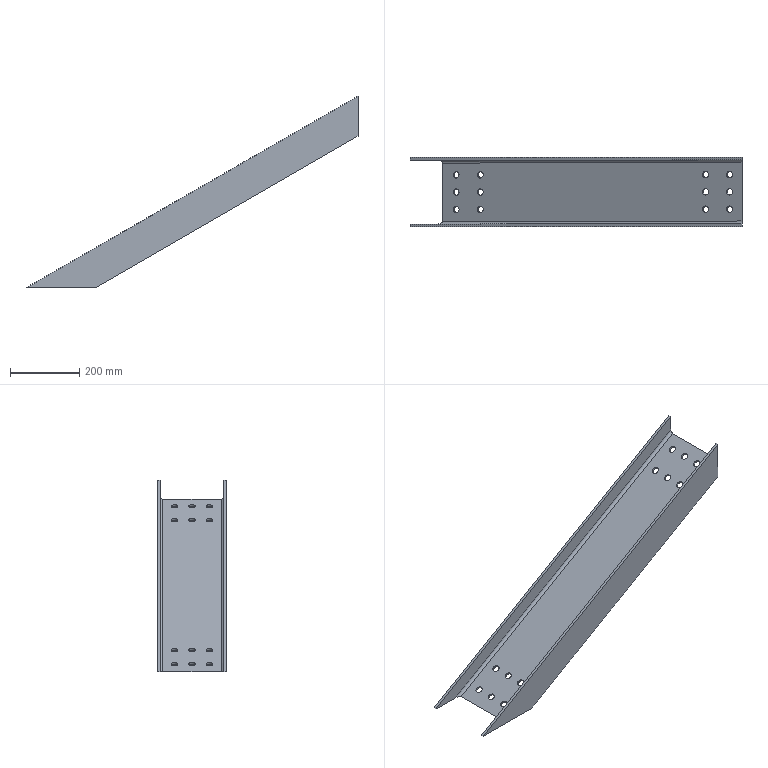Part | STEP file | 粉仓Diagonal Brace梁2_Default<As Machined> | 1 solid | 42 faces | box 957.365 x 200 x 552.735 mm | volume 2621556 mm3 | cylinder 28 | plane 14 | commonest cylinder face diameters 19 x24 16 x4